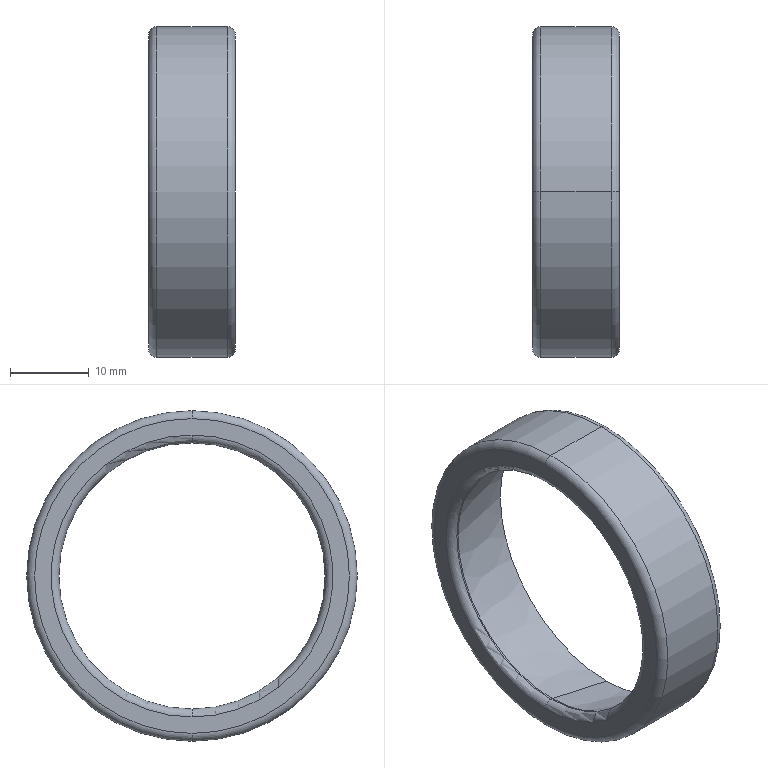Part | NX | features BREP 1 | 1 solid | 14 faces | box 11 x 42 x 42 mm | volume 4079 mm3 | torus 8 | plane 2 | cylinder 2 | cone 2 | commonest cylinder face diameters 42 x2
STEP:
#1=CARTESIAN_POINT('',(-0.25,0.,-16.908));
#2=VERTEX_POINT('',#1);
#3=CARTESIAN_POINT('',(-0.03356,0.,-16.932));
#4=VERTEX_POINT('',#3);
#5=CARTESIAN_POINT('',(-0.25,0.,-17.908));
#6=DIRECTION('',(0.,1.,0.));
#7=DIRECTION('',(0.,0.,1.));
#8=AXIS2_PLACEMENT_3D('',#5,#6,#7);
#9=CIRCLE('',#8,1.);
#10=EDGE_CURVE('',#2,#4,#9,.T.);
#11=ORIENTED_EDGE('',*,*,#10,.T.);
#12=CARTESIAN_POINT('',(-0.03356,0.,16.932));
#13=VERTEX_POINT('',#12);
#14=CARTESIAN_POINT('',(-0.03356,0.,0.));
#15=DIRECTION('',(1.,0.,0.));
#16=DIRECTION('',(0.,0.,-1.));
#17=AXIS2_PLACEMENT_3D('',#14,#15,#16);
#18=CIRCLE('',#17,16.932);
#19=EDGE_CURVE('',#4,#13,#18,.T.);
#20=ORIENTED_EDGE('',*,*,#19,.T.);
#21=CARTESIAN_POINT('',(-0.25,0.,16.908));
#22=VERTEX_POINT('',#21);
#23=CARTESIAN_POINT('',(-0.25,0.,17.908));
#24=DIRECTION('',(0.,-1.,0.));
#25=DIRECTION('',(0.,0.,-1.));
#26=AXIS2_PLACEMENT_3D('',#23,#24,#25);
#27=CIRCLE('',#26,1.);
#28=EDGE_CURVE('',#22,#13,#27,.T.);
#29=ORIENTED_EDGE('',*,*,#28,.F.);
#30=CARTESIAN_POINT('',(-0.25,0.,0.));
#31=DIRECTION('',(-1.,0.,0.));
#32=DIRECTION('',(0.,0.,1.));
#33=AXIS2_PLACEMENT_3D('',#30,#31,#32);
#34=CIRCLE('',#33,16.908);
#35=EDGE_CURVE('',#22,#2,#34,.T.);
#36=ORIENTED_EDGE('',*,*,#35,.T.);
#37=EDGE_LOOP('',(#11,#20,#29,#36));
#38=FACE_BOUND('',#37,.T.);
#39=CARTESIAN_POINT('',(-0.25,0.,0.));
#40=DIRECTION('',(1.,0.,0.));
#41=DIRECTION('',(0.,0.,-1.));
#42=AXIS2_PLACEMENT_3D('',#39,#40,#41);
#43=TOROIDAL_SURFACE('',#42,17.908,1.);
#44=ADVANCED_FACE('',(#38),#43,.T.);
#45=ORIENTED_EDGE('',*,*,#35,.F.);
#46=CARTESIAN_POINT('',(-1.25,0.,17.908));
#47=VERTEX_POINT('',#46);
#48=CARTESIAN_POINT('',(-0.25,0.,17.908));
#49=DIRECTION('',(0.,-1.,0.));
#50=DIRECTION('',(-1.,0.,0.));
#51=AXIS2_PLACEMENT_3D('',#48,#49,#50);
#52=CIRCLE('',#51,1.);
#53=EDGE_CURVE('',#22,#47,#52,.F.);
#54=ORIENTED_EDGE('',*,*,#53,.T.);
#55=CARTESIAN_POINT('',(-1.25,0.,-17.908));
#56=VERTEX_POINT('',#55);
#57=CARTESIAN_POINT('',(-1.25,0.,0.));
#58=DIRECTION('',(1.,0.,0.));
#59=DIRECTION('',(0.,0.,-1.));
#60=AXIS2_PLACEMENT_3D('',#57,#58,#59);
#61=CIRCLE('',#60,17.908);
#62=EDGE_CURVE('',#56,#47,#61,.T.);
#63=ORIENTED_EDGE('',*,*,#62,.F.);
#64=CARTESIAN_POINT('',(-0.25,0.,-17.908));
#65=DIRECTION('',(0.,1.,0.));
#66=DIRECTION('',(-1.,0.,0.));
#67=AXIS2_PLACEMENT_3D('',#64,#65,#66);
#68=CIRCLE('',#67,1.);
#69=EDGE_CURVE('',#2,#56,#68,.F.);
#70=ORIENTED_EDGE('',*,*,#69,.F.);
#71=EDGE_LOOP('',(#45,#54,#63,#70));
#72=FACE_BOUND('',#71,.T.);
#73=CARTESIAN_POINT('',(-0.25,0.,0.));
#74=DIRECTION('',(1.,0.,0.));
#75=DIRECTION('',(0.,0.,-1.));
#76=AXIS2_PLACEMENT_3D('',#73,#74,#75);
#77=TOROIDAL_SURFACE('',#76,17.908,1.);
#78=ADVANCED_FACE('',(#72),#77,.T.);
#79=CARTESIAN_POINT('',(-0.25,0.,0.));
#80=DIRECTION('',(-1.,0.,0.));
#81=DIRECTION('',(0.,0.,-1.));
#82=AXIS2_PLACEMENT_3D('',#79,#80,#81);
#83=CIRCLE('',#82,16.908);
#84=EDGE_CURVE('',#2,#22,#83,.T.);
#85=ORIENTED_EDGE('',*,*,#84,.F.);
#86=ORIENTED_EDGE('',*,*,#69,.T.);
#87=CARTESIAN_POINT('',(-1.25,0.,0.));
#88=DIRECTION('',(1.,0.,0.));
#89=DIRECTION('',(0.,0.,1.));
#90=AXIS2_PLACEMENT_3D('',#87,#88,#89);
#91=CIRCLE('',#90,17.908);
#92=EDGE_CURVE('',#47,#56,#91,.T.);
#93=ORIENTED_EDGE('',*,*,#92,.F.);
#94=ORIENTED_EDGE('',*,*,#53,.F.);
#95=EDGE_LOOP('',(#85,#86,#93,#94));
#96=FACE_BOUND('',#95,.T.);
#97=CARTESIAN_POINT('',(-0.25,0.,0.));
#98=DIRECTION('',(1.,0.,0.));
#99=DIRECTION('',(0.,0.,-1.));
#100=AXIS2_PLACEMENT_3D('',#97,#98,#99);
#101=TOROIDAL_SURFACE('',#100,17.908,1.);
#102=ADVANCED_FACE('',(#96),#101,.T.);
#103=CARTESIAN_POINT('',(-1.25,0.,20.));
#104=VERTEX_POINT('',#103);
#105=CARTESIAN_POINT('',(-1.25,0.,-20.));
#106=VERTEX_POINT('',#105);
#107=CARTESIAN_POINT('',(-1.25,0.,0.));
#108=DIRECTION('',(-1.,0.,0.));
#109=DIRECTION('',(0.,0.,1.));
#110=AXIS2_PLACEMENT_3D('',#107,#108,#109);
#111=CIRCLE('',#110,20.);
#112=EDGE_CURVE('',#104,#106,#111,.T.);
#113=ORIENTED_EDGE('',*,*,#112,.T.);
#114=CARTESIAN_POINT('',(-1.25,0.,0.));
#115=DIRECTION('',(-1.,0.,0.));
#116=DIRECTION('',(0.,0.,-1.));
#117=AXIS2_PLACEMENT_3D('',#114,#115,#116);
#118=CIRCLE('',#117,20.);
#119=EDGE_CURVE('',#106,#104,#118,.T.);
#120=ORIENTED_EDGE('',*,*,#119,.T.);
#121=EDGE_LOOP('',(#113,#120));
#122=FACE_BOUND('',#121,.T.);
#123=ORIENTED_EDGE('',*,*,#92,.T.);
#124=ORIENTED_EDGE('',*,*,#62,.T.);
#125=EDGE_LOOP('',(#123,#124));
#126=FACE_BOUND('',#125,.T.);
#127=CARTESIAN_POINT('',(-1.25,16.662,0.));
#128=DIRECTION('',(1.,0.,0.));
#129=DIRECTION('',(0.,1.,0.));
#130=AXIS2_PLACEMENT_3D('',#127,#128,#129);
#131=PLANE('',#130);
#132=ADVANCED_FACE('',(#122,#126),#131,.F.);
#133=ORIENTED_EDGE('',*,*,#119,.F.);
#134=CARTESIAN_POINT('',(-0.25,0.,-21.));
#135=VERTEX_POINT('',#134);
#136=CARTESIAN_POINT('',(-0.25,0.,-20.));
#137=DIRECTION('',(0.,1.,0.));
#138=DIRECTION('',(0.,0.,-1.));
#139=AXIS2_PLACEMENT_3D('',#136,#137,#138);
#140=CIRCLE('',#139,1.);
#141=EDGE_CURVE('',#135,#106,#140,.T.);
#142=ORIENTED_EDGE('',*,*,#141,.F.);
#143=CARTESIAN_POINT('',(-0.25,0.,21.));
#144=VERTEX_POINT('',#143);
#145=CARTESIAN_POINT('',(-0.25,0.,0.));
#146=DIRECTION('',(-1.,0.,0.));
#147=DIRECTION('',(0.,0.,-1.));
#148=AXIS2_PLACEMENT_3D('',#145,#146,#147);
#149=CIRCLE('',#148,21.);
#150=EDGE_CURVE('',#135,#144,#149,.T.);
#151=ORIENTED_EDGE('',*,*,#150,.T.);
#152=CARTESIAN_POINT('',(-0.25,0.,20.));
#153=DIRECTION('',(0.,-1.,0.));
#154=DIRECTION('',(0.,0.,1.));
#155=AXIS2_PLACEMENT_3D('',#152,#153,#154);
#156=CIRCLE('',#155,1.);
#157=EDGE_CURVE('',#144,#104,#156,.T.);
#158=ORIENTED_EDGE('',*,*,#157,.T.);
#159=EDGE_LOOP('',(#133,#142,#151,#158));
#160=FACE_BOUND('',#159,.T.);
#161=CARTESIAN_POINT('',(-0.25,0.,0.));
#162=DIRECTION('',(1.,0.,0.));
#163=DIRECTION('',(0.,0.,-1.));
#164=AXIS2_PLACEMENT_3D('',#161,#162,#163);
#165=TOROIDAL_SURFACE('',#164,20.,1.);
#166=ADVANCED_FACE('',(#160),#165,.T.);
#167=ORIENTED_EDGE('',*,*,#157,.F.);
#168=CARTESIAN_POINT('',(-0.25,0.,0.));
#169=DIRECTION('',(-1.,0.,0.));
#170=DIRECTION('',(0.,0.,1.));
#171=AXIS2_PLACEMENT_3D('',#168,#169,#170);
#172=CIRCLE('',#171,21.);
#173=EDGE_CURVE('',#144,#135,#172,.T.);
#174=ORIENTED_EDGE('',*,*,#173,.T.);
#175=ORIENTED_EDGE('',*,*,#141,.T.);
#176=ORIENTED_EDGE('',*,*,#112,.F.);
#177=EDGE_LOOP('',(#167,#174,#175,#176));
#178=FACE_BOUND('',#177,.T.);
#179=CARTESIAN_POINT('',(-0.25,0.,0.));
#180=DIRECTION('',(1.,0.,0.));
#181=DIRECTION('',(0.,0.,-1.));
#182=AXIS2_PLACEMENT_3D('',#179,#180,#181);
#183=TOROIDAL_SURFACE('',#182,20.,1.);
#184=ADVANCED_FACE('',(#178),#183,.T.);
#185=CARTESIAN_POINT('',(8.75,0.,-21.));
#186=VERTEX_POINT('',#185);
#187=CARTESIAN_POINT('',(-0.25,0.,-21.));
#188=DIRECTION('',(1.,0.,0.));
#189=VECTOR('',#188,1000.);
#190=LINE('',#187,#189);
#191=EDGE_CURVE('',#135,#186,#190,.T.);
#192=ORIENTED_EDGE('',*,*,#191,.F.);
#193=ORIENTED_EDGE('',*,*,#173,.F.);
#194=CARTESIAN_POINT('',(8.75,0.,21.));
#195=VERTEX_POINT('',#194);
#196=CARTESIAN_POINT('',(-0.25,0.,21.));
#197=DIRECTION('',(1.,0.,0.));
#198=VECTOR('',#197,1000.);
#199=LINE('',#196,#198);
#200=EDGE_CURVE('',#144,#195,#199,.T.);
#201=ORIENTED_EDGE('',*,*,#200,.T.);
#202=CARTESIAN_POINT('',(8.75,0.,0.));
#203=DIRECTION('',(1.,0.,0.));
#204=DIRECTION('',(0.,0.,-1.));
#205=AXIS2_PLACEMENT_3D('',#202,#203,#204);
#206=CIRCLE('',#205,21.);
#207=EDGE_CURVE('',#186,#195,#206,.T.);
#208=ORIENTED_EDGE('',*,*,#207,.F.);
#209=EDGE_LOOP('',(#192,#193,#201,#208));
#210=FACE_BOUND('',#209,.T.);
#211=CARTESIAN_POINT('',(0.,0.,0.));
#212=DIRECTION('',(-1.,0.,0.));
#213=DIRECTION('',(0.,0.,1.));
#214=AXIS2_PLACEMENT_3D('',#211,#212,#213);
#215=CYLINDRICAL_SURFACE('',#214,21.);
#216=ADVANCED_FACE('',(#210),#215,.T.);
#217=CARTESIAN_POINT('',(9.75,0.,-20.));
#218=VERTEX_POINT('',#217);
#219=CARTESIAN_POINT('',(8.75,0.,-20.));
#220=DIRECTION('',(0.,-1.,0.));
#221=DIRECTION('',(0.,0.,-1.));
#222=AXIS2_PLACEMENT_3D('',#219,#220,#221);
#223=CIRCLE('',#222,1.);
#224=EDGE_CURVE('',#186,#218,#223,.T.);
#225=ORIENTED_EDGE('',*,*,#224,.F.);
#226=ORIENTED_EDGE('',*,*,#207,.T.);
#227=CARTESIAN_POINT('',(9.75,0.,20.));
#228=VERTEX_POINT('',#227);
#229=CARTESIAN_POINT('',(8.75,0.,20.));
#230=DIRECTION('',(0.,1.,0.));
#231=DIRECTION('',(0.,0.,1.));
#232=AXIS2_PLACEMENT_3D('',#229,#230,#231);
#233=CIRCLE('',#232,1.);
#234=EDGE_CURVE('',#195,#228,#233,.T.);
#235=ORIENTED_EDGE('',*,*,#234,.T.);
#236=CARTESIAN_POINT('',(9.75,0.,0.));
#237=DIRECTION('',(1.,0.,0.));
#238=DIRECTION('',(0.,0.,-1.));
#239=AXIS2_PLACEMENT_3D('',#236,#237,#238);
#240=CIRCLE('',#239,20.);
#241=EDGE_CURVE('',#218,#228,#240,.T.);
#242=ORIENTED_EDGE('',*,*,#241,.F.);
#243=EDGE_LOOP('',(#225,#226,#235,#242));
#244=FACE_BOUND('',#243,.T.);
#245=CARTESIAN_POINT('',(8.75,0.,0.));
#246=DIRECTION('',(-1.,0.,0.));
#247=DIRECTION('',(0.,0.,1.));
#248=AXIS2_PLACEMENT_3D('',#245,#246,#247);
#249=TOROIDAL_SURFACE('',#248,20.,1.);
#250=ADVANCED_FACE('',(#244),#249,.T.);
#251=ORIENTED_EDGE('',*,*,#241,.T.);
#252=CARTESIAN_POINT('',(9.75,0.,0.));
#253=DIRECTION('',(1.,0.,0.));
#254=DIRECTION('',(0.,0.,1.));
#255=AXIS2_PLACEMENT_3D('',#252,#253,#254);
#256=CIRCLE('',#255,20.);
#257=EDGE_CURVE('',#228,#218,#256,.T.);
#258=ORIENTED_EDGE('',*,*,#257,.T.);
#259=EDGE_LOOP('',(#251,#258));
#260=FACE_BOUND('',#259,.T.);
#261=CARTESIAN_POINT('',(9.75,0.,19.101));
#262=VERTEX_POINT('',#261);
#263=CARTESIAN_POINT('',(9.75,0.,-19.101));
#264=VERTEX_POINT('',#263);
#265=CARTESIAN_POINT('',(9.75,0.,0.));
#266=DIRECTION('',(-1.,0.,0.));
#267=DIRECTION('',(0.,0.,1.));
#268=AXIS2_PLACEMENT_3D('',#265,#266,#267);
#269=CIRCLE('',#268,19.101);
#270=EDGE_CURVE('',#262,#264,#269,.T.);
#271=ORIENTED_EDGE('',*,*,#270,.T.);
#272=CARTESIAN_POINT('',(9.75,0.,0.));
#273=DIRECTION('',(-1.,0.,0.));
#274=DIRECTION('',(0.,0.,-1.));
#275=AXIS2_PLACEMENT_3D('',#272,#273,#274);
#276=CIRCLE('',#275,19.101);
#277=EDGE_CURVE('',#264,#262,#276,.T.);
#278=ORIENTED_EDGE('',*,*,#277,.T.);
#279=EDGE_LOOP('',(#271,#278));
#280=FACE_BOUND('',#279,.T.);
#281=CARTESIAN_POINT('',(9.75,21.,0.));
#282=DIRECTION('',(-1.,0.,0.));
#283=DIRECTION('',(0.,0.,1.));
#284=AXIS2_PLACEMENT_3D('',#281,#282,#283);
#285=PLANE('',#284);
#286=ADVANCED_FACE('',(#260,#280),#285,.F.);
#287=ORIENTED_EDGE('',*,*,#257,.F.);
#288=ORIENTED_EDGE('',*,*,#234,.F.);
#289=CARTESIAN_POINT('',(8.75,0.,0.));
#290=DIRECTION('',(1.,0.,0.));
#291=DIRECTION('',(0.,0.,1.));
#292=AXIS2_PLACEMENT_3D('',#289,#290,#291);
#293=CIRCLE('',#292,21.);
#294=EDGE_CURVE('',#195,#186,#293,.T.);
#295=ORIENTED_EDGE('',*,*,#294,.T.);
#296=ORIENTED_EDGE('',*,*,#224,.T.);
#297=EDGE_LOOP('',(#287,#288,#295,#296));
#298=FACE_BOUND('',#297,.T.);
#299=CARTESIAN_POINT('',(8.75,0.,0.));
#300=DIRECTION('',(-1.,0.,0.));
#301=DIRECTION('',(0.,0.,1.));
#302=AXIS2_PLACEMENT_3D('',#299,#300,#301);
#303=TOROIDAL_SURFACE('',#302,20.,1.);
#304=ADVANCED_FACE('',(#298),#303,.T.);
#305=ORIENTED_EDGE('',*,*,#294,.F.);
#306=ORIENTED_EDGE('',*,*,#200,.F.);
#307=ORIENTED_EDGE('',*,*,#150,.F.);
#308=ORIENTED_EDGE('',*,*,#191,.T.);
#309=EDGE_LOOP('',(#305,#306,#307,#308));
#310=FACE_BOUND('',#309,.T.);
#311=CARTESIAN_POINT('',(0.,0.,0.));
#312=DIRECTION('',(-1.,0.,0.));
#313=DIRECTION('',(0.,0.,1.));
#314=AXIS2_PLACEMENT_3D('',#311,#312,#313);
#315=CYLINDRICAL_SURFACE('',#314,21.);
#316=ADVANCED_FACE('',(#310),#315,.T.);
#317=CARTESIAN_POINT('',(9.75,0.,19.101));
#318=DIRECTION('',(-0.9763,0.,-0.2164));
#319=VECTOR('',#318,1000.);
#320=LINE('',#317,#319);
#321=EDGE_CURVE('',#13,#262,#320,.F.);
#322=ORIENTED_EDGE('',*,*,#321,.T.);
#323=ORIENTED_EDGE('',*,*,#277,.F.);
#324=CARTESIAN_POINT('',(9.75,0.,-19.101));
#325=DIRECTION('',(-0.9763,0.,0.2164));
#326=VECTOR('',#325,1000.);
#327=LINE('',#324,#326);
#328=EDGE_CURVE('',#4,#264,#327,.F.);
#329=ORIENTED_EDGE('',*,*,#328,.F.);
#330=CARTESIAN_POINT('',(-0.03356,0.,0.));
#331=DIRECTION('',(1.,0.,0.));
#332=DIRECTION('',(0.,0.,1.));
#333=AXIS2_PLACEMENT_3D('',#330,#331,#332);
#334=CIRCLE('',#333,16.932);
#335=EDGE_CURVE('',#13,#4,#334,.T.);
#336=ORIENTED_EDGE('',*,*,#335,.F.);
#337=EDGE_LOOP('',(#322,#323,#329,#336));
#338=FACE_BOUND('',#337,.T.);
#339=CARTESIAN_POINT('',(4.858,0.,0.));
#340=DIRECTION('',(1.,0.,0.));
#341=DIRECTION('',(0.,0.,-1.));
#342=AXIS2_PLACEMENT_3D('',#339,#340,#341);
#343=CONICAL_SURFACE('',#342,18.016,0.2182);
#344=ADVANCED_FACE('',(#338),#343,.F.);
#345=ORIENTED_EDGE('',*,*,#28,.T.);
#346=ORIENTED_EDGE('',*,*,#335,.T.);
#347=ORIENTED_EDGE('',*,*,#10,.F.);
#348=ORIENTED_EDGE('',*,*,#84,.T.);
#349=EDGE_LOOP('',(#345,#346,#347,#348));
#350=FACE_BOUND('',#349,.T.);
#351=CARTESIAN_POINT('',(-0.25,0.,0.));
#352=DIRECTION('',(1.,0.,0.));
#353=DIRECTION('',(0.,0.,-1.));
#354=AXIS2_PLACEMENT_3D('',#351,#352,#353);
#355=TOROIDAL_SURFACE('',#354,17.908,1.);
#356=ADVANCED_FACE('',(#350),#355,.T.);
#357=ORIENTED_EDGE('',*,*,#19,.F.);
#358=ORIENTED_EDGE('',*,*,#328,.T.);
#359=ORIENTED_EDGE('',*,*,#270,.F.);
#360=ORIENTED_EDGE('',*,*,#321,.F.);
#361=EDGE_LOOP('',(#357,#358,#359,#360));
#362=FACE_BOUND('',#361,.T.);
#363=CARTESIAN_POINT('',(4.858,0.,0.));
#364=DIRECTION('',(1.,0.,0.));
#365=DIRECTION('',(0.,0.,-1.));
#366=AXIS2_PLACEMENT_3D('',#363,#364,#365);
#367=CONICAL_SURFACE('',#366,18.016,0.2182);
#368=ADVANCED_FACE('',(#362),#367,.F.);
#369=CLOSED_SHELL('',(#44,#78,#102,#132,#166,#184,#216,#250,#286,#304,#316,#344,#356,#368));
#370=MANIFOLD_SOLID_BREP('',#369);
#371=(LENGTH_UNIT()NAMED_UNIT(*)SI_UNIT(.MILLI.,.METRE.));
#372=UNCERTAINTY_MEASURE_WITH_UNIT(LENGTH_MEASURE(0.00001),#371,'','');
#373=(NAMED_UNIT(*)PLANE_ANGLE_UNIT()SI_UNIT($,.RADIAN.));
#374=(NAMED_UNIT(*)SI_UNIT($,.STERADIAN.)SOLID_ANGLE_UNIT());
#375=(GEOMETRIC_REPRESENTATION_CONTEXT(3)GLOBAL_UNCERTAINTY_ASSIGNED_CONTEXT((#372))GLOBAL_UNIT_ASSIGNED_CONTEXT((#371,#373,#374))REPRESENTATION_CONTEXT('',''));
#376=ADVANCED_BREP_SHAPE_REPRESENTATION('',(#370),#375);